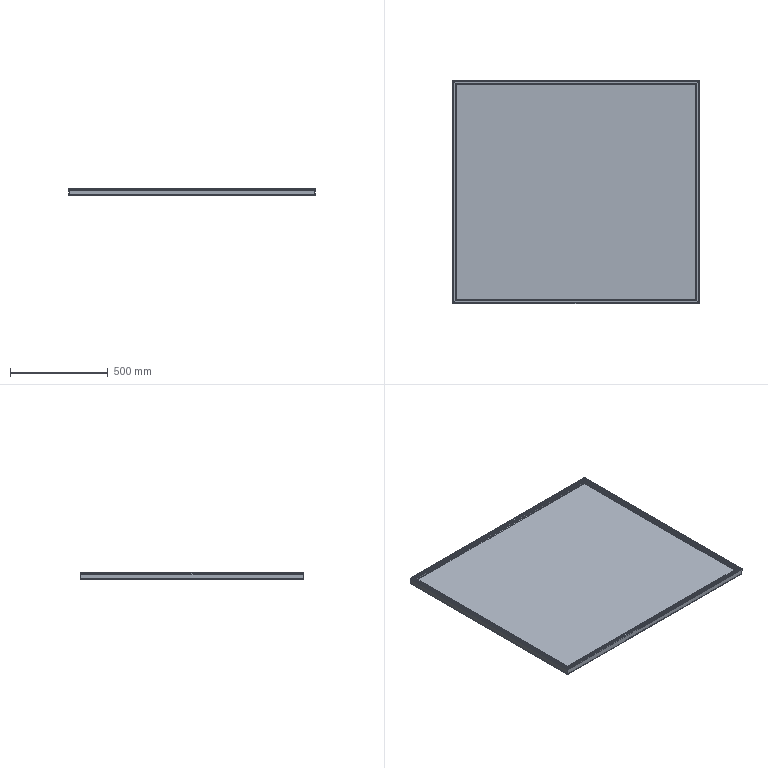Part | SolidWorks | features ICE 1, WeldMemberFeat 1, WeldmentFeature 1 | 5 solids | 94 faces | box 1260 x 1140 x 35 mm | volume 4920014 mm3 | plane 86 | cylinder 8 | commonest cylinder face diameters 1 x4 2 x4